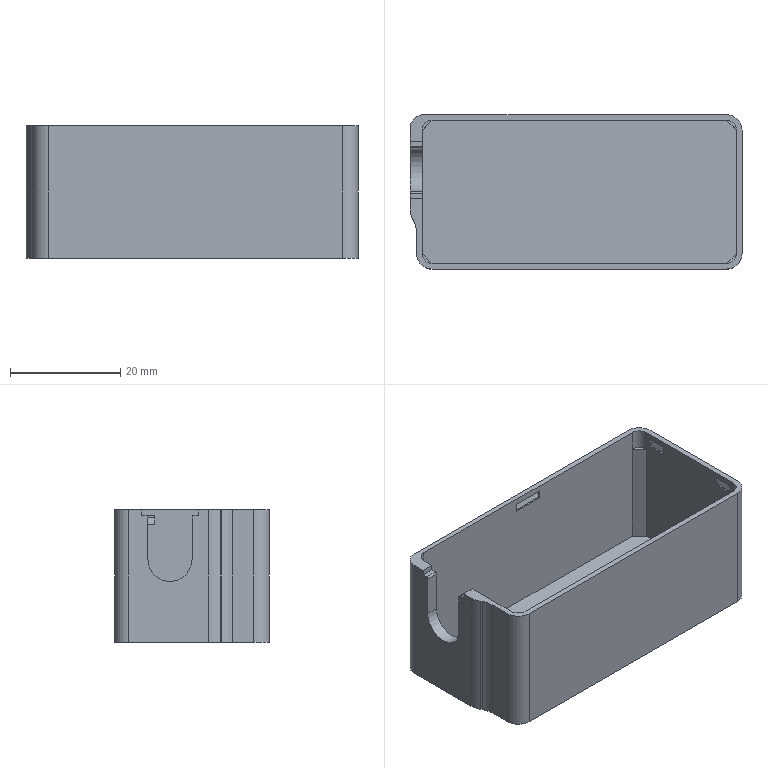Part | SolidWorks | features ICE 9, MirrorPattern 3, Cut 1, DelFace 1, Extrusion 1, Fillet 1 | 1 solid | 70 faces | box 60.2 x 28 x 24 mm | volume 5859 mm3 | plane 57 | cylinder 13 | commonest cylinder face diameters 3.6 x4 5.6 x3 8 x3 0.6 x2 5 x1